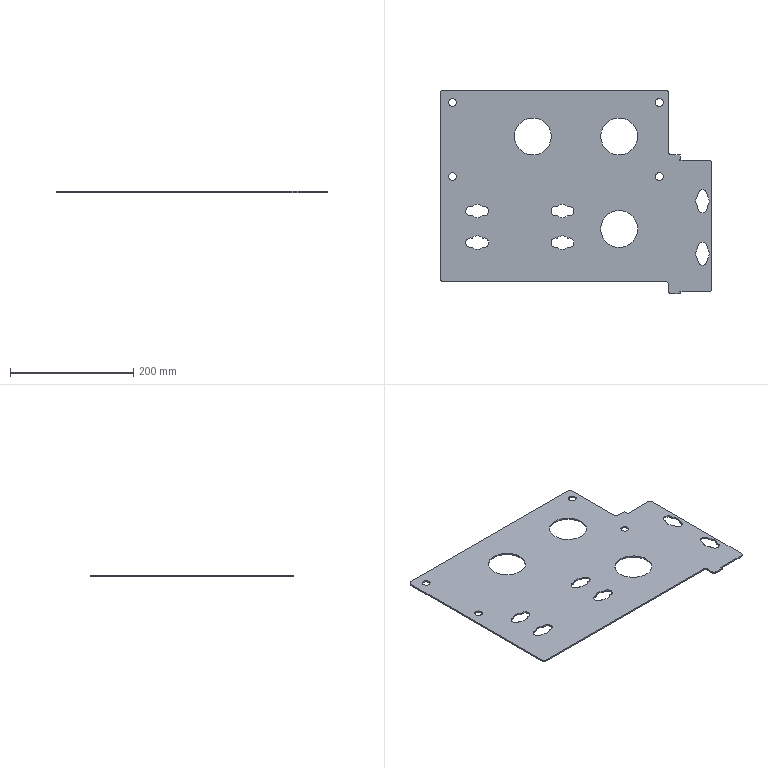Part | SolidWorks | features FlatPattern 1, SMBaseFlange 1, SheetMetal 1 | 1 solid | 110 faces | box 440 x 330 x 2.3 mm | volume 269953 mm3 | cylinder 96 | plane 14 | commonest cylinder face diameters 4 x28 15 x24 22 x14 10 x8 12.5 x8 60 x6